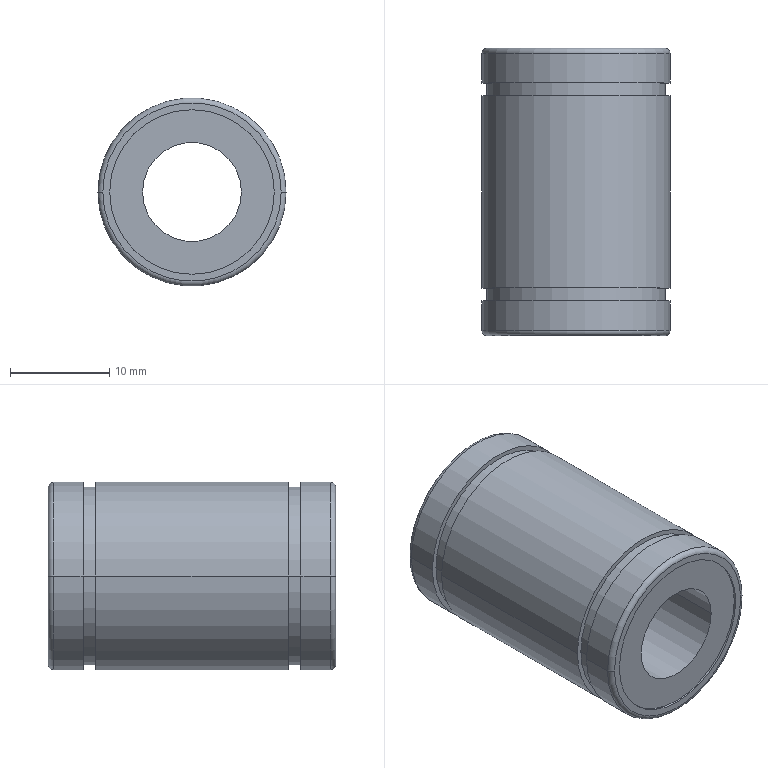Part | NX | 1 solid | 28 faces | box 19 x 29 x 19 mm | volume 5808 mm3 | cylinder 16 | plane 8 | torus 4 | commonest cylinder face diameters 19 x6 16.6 x4 18 x4 10 x2
STEP:
#1=CARTESIAN_POINT('',(-5.,-14.3,0.));
#2=VERTEX_POINT('',#1);
#3=CARTESIAN_POINT('',(5.,-14.3,0.));
#4=VERTEX_POINT('',#3);
#5=CARTESIAN_POINT('',(0.,-14.3,0.));
#6=DIRECTION('',(0.,1.,0.));
#7=DIRECTION('',(-1.,0.,0.));
#8=AXIS2_PLACEMENT_3D('',#5,#6,#7);
#9=CIRCLE('',#8,5.);
#10=EDGE_CURVE('',#2,#4,#9,.T.);
#11=ORIENTED_EDGE('',*,*,#10,.F.);
#12=CARTESIAN_POINT('',(-5.,14.3,0.));
#13=VERTEX_POINT('',#12);
#14=CARTESIAN_POINT('',(-5.,-15.95,0.));
#15=DIRECTION('',(0.,1.,0.));
#16=VECTOR('',#15,1000.);
#17=LINE('',#14,#16);
#18=EDGE_CURVE('',#2,#13,#17,.T.);
#19=ORIENTED_EDGE('',*,*,#18,.T.);
#20=CARTESIAN_POINT('',(5.,14.3,0.));
#21=VERTEX_POINT('',#20);
#22=CARTESIAN_POINT('',(0.,14.3,0.));
#23=DIRECTION('',(0.,-1.,0.));
#24=DIRECTION('',(1.,0.,0.));
#25=AXIS2_PLACEMENT_3D('',#22,#23,#24);
#26=CIRCLE('',#25,5.);
#27=EDGE_CURVE('',#21,#13,#26,.T.);
#28=ORIENTED_EDGE('',*,*,#27,.F.);
#29=CARTESIAN_POINT('',(5.,-15.95,0.));
#30=DIRECTION('',(0.,1.,0.));
#31=VECTOR('',#30,1000.);
#32=LINE('',#29,#31);
#33=EDGE_CURVE('',#4,#21,#32,.T.);
#34=ORIENTED_EDGE('',*,*,#33,.F.);
#35=EDGE_LOOP('',(#11,#19,#28,#34));
#36=FACE_BOUND('',#35,.T.);
#37=CARTESIAN_POINT('',(0.,-15.95,0.));
#38=DIRECTION('',(0.,1.,0.));
#39=DIRECTION('',(1.,0.,0.));
#40=AXIS2_PLACEMENT_3D('',#37,#38,#39);
#41=CYLINDRICAL_SURFACE('',#40,5.);
#42=ADVANCED_FACE('',(#36),#41,.F.);
#43=CARTESIAN_POINT('',(-8.3,14.3,0.));
#44=VERTEX_POINT('',#43);
#45=CARTESIAN_POINT('',(8.3,14.3,0.));
#46=VERTEX_POINT('',#45);
#47=CARTESIAN_POINT('',(0.,14.3,0.));
#48=DIRECTION('',(0.,1.,0.));
#49=DIRECTION('',(1.,0.,0.));
#50=AXIS2_PLACEMENT_3D('',#47,#48,#49);
#51=CIRCLE('',#50,8.3);
#52=EDGE_CURVE('',#44,#46,#51,.T.);
#53=ORIENTED_EDGE('',*,*,#52,.T.);
#54=CARTESIAN_POINT('',(0.,14.3,0.));
#55=DIRECTION('',(0.,1.,0.));
#56=DIRECTION('',(1.,0.,0.));
#57=AXIS2_PLACEMENT_3D('',#54,#55,#56);
#58=CIRCLE('',#57,8.3);
#59=EDGE_CURVE('',#46,#44,#58,.T.);
#60=ORIENTED_EDGE('',*,*,#59,.T.);
#61=EDGE_LOOP('',(#53,#60));
#62=FACE_BOUND('',#61,.T.);
#63=ORIENTED_EDGE('',*,*,#27,.T.);
#64=CARTESIAN_POINT('',(0.,14.3,0.));
#65=DIRECTION('',(0.,-1.,0.));
#66=DIRECTION('',(1.,0.,0.));
#67=AXIS2_PLACEMENT_3D('',#64,#65,#66);
#68=CIRCLE('',#67,5.);
#69=EDGE_CURVE('',#13,#21,#68,.T.);
#70=ORIENTED_EDGE('',*,*,#69,.T.);
#71=EDGE_LOOP('',(#63,#70));
#72=FACE_BOUND('',#71,.T.);
#73=CARTESIAN_POINT('',(0.,14.3,0.));
#74=DIRECTION('',(0.,1.,0.));
#75=DIRECTION('',(1.,0.,0.));
#76=AXIS2_PLACEMENT_3D('',#73,#74,#75);
#77=PLANE('',#76);
#78=ADVANCED_FACE('',(#62,#72),#77,.T.);
#79=ORIENTED_EDGE('',*,*,#52,.F.);
#80=CARTESIAN_POINT('',(-8.3,14.5,0.));
#81=VERTEX_POINT('',#80);
#82=CARTESIAN_POINT('',(-8.3,14.5,0.));
#83=DIRECTION('',(0.,-1.,0.));
#84=VECTOR('',#83,1000.);
#85=LINE('',#82,#84);
#86=EDGE_CURVE('',#44,#81,#85,.F.);
#87=ORIENTED_EDGE('',*,*,#86,.T.);
#88=CARTESIAN_POINT('',(8.3,14.5,0.));
#89=VERTEX_POINT('',#88);
#90=CARTESIAN_POINT('',(0.,14.5,0.));
#91=DIRECTION('',(0.,-1.,0.));
#92=DIRECTION('',(-1.,0.,0.));
#93=AXIS2_PLACEMENT_3D('',#90,#91,#92);
#94=CIRCLE('',#93,8.3);
#95=EDGE_CURVE('',#89,#81,#94,.T.);
#96=ORIENTED_EDGE('',*,*,#95,.F.);
#97=CARTESIAN_POINT('',(8.3,14.5,0.));
#98=DIRECTION('',(0.,-1.,0.));
#99=VECTOR('',#98,1000.);
#100=LINE('',#97,#99);
#101=EDGE_CURVE('',#46,#89,#100,.F.);
#102=ORIENTED_EDGE('',*,*,#101,.F.);
#103=EDGE_LOOP('',(#79,#87,#96,#102));
#104=FACE_BOUND('',#103,.T.);
#105=CARTESIAN_POINT('',(0.,14.5,0.));
#106=DIRECTION('',(0.,-1.,0.));
#107=DIRECTION('',(-1.,0.,0.));
#108=AXIS2_PLACEMENT_3D('',#105,#106,#107);
#109=CYLINDRICAL_SURFACE('',#108,8.3);
#110=ADVANCED_FACE('',(#104),#109,.F.);
#111=CARTESIAN_POINT('',(-9.,14.5,0.));
#112=VERTEX_POINT('',#111);
#113=CARTESIAN_POINT('',(9.,14.5,0.));
#114=VERTEX_POINT('',#113);
#115=CARTESIAN_POINT('',(0.,14.5,0.));
#116=DIRECTION('',(0.,-1.,0.));
#117=DIRECTION('',(1.,0.,0.));
#118=AXIS2_PLACEMENT_3D('',#115,#116,#117);
#119=CIRCLE('',#118,9.);
#120=EDGE_CURVE('',#112,#114,#119,.T.);
#121=ORIENTED_EDGE('',*,*,#120,.F.);
#122=CARTESIAN_POINT('',(0.,14.5,0.));
#123=DIRECTION('',(0.,-1.,0.));
#124=DIRECTION('',(1.,0.,0.));
#125=AXIS2_PLACEMENT_3D('',#122,#123,#124);
#126=CIRCLE('',#125,9.);
#127=EDGE_CURVE('',#114,#112,#126,.T.);
#128=ORIENTED_EDGE('',*,*,#127,.F.);
#129=EDGE_LOOP('',(#121,#128));
#130=FACE_BOUND('',#129,.T.);
#131=CARTESIAN_POINT('',(0.,14.5,0.));
#132=DIRECTION('',(0.,-1.,0.));
#133=DIRECTION('',(-1.,0.,0.));
#134=AXIS2_PLACEMENT_3D('',#131,#132,#133);
#135=CIRCLE('',#134,8.3);
#136=EDGE_CURVE('',#81,#89,#135,.T.);
#137=ORIENTED_EDGE('',*,*,#136,.T.);
#138=ORIENTED_EDGE('',*,*,#95,.T.);
#139=EDGE_LOOP('',(#137,#138));
#140=FACE_BOUND('',#139,.T.);
#141=CARTESIAN_POINT('',(0.,14.5,0.));
#142=DIRECTION('',(0.,-1.,0.));
#143=DIRECTION('',(0.,0.,-1.));
#144=AXIS2_PLACEMENT_3D('',#141,#142,#143);
#145=PLANE('',#144);
#146=ADVANCED_FACE('',(#130,#140),#145,.F.);
#147=CARTESIAN_POINT('',(-9.5,14.,0.));
#148=VERTEX_POINT('',#147);
#149=CARTESIAN_POINT('',(9.5,14.,0.));
#150=VERTEX_POINT('',#149);
#151=CARTESIAN_POINT('',(0.,14.,0.));
#152=DIRECTION('',(0.,-1.,0.));
#153=DIRECTION('',(1.,0.,0.));
#154=AXIS2_PLACEMENT_3D('',#151,#152,#153);
#155=CIRCLE('',#154,9.5);
#156=EDGE_CURVE('',#148,#150,#155,.T.);
#157=ORIENTED_EDGE('',*,*,#156,.F.);
#158=CARTESIAN_POINT('',(-9.,14.,0.));
#159=DIRECTION('',(0.,0.,1.));
#160=DIRECTION('',(-1.,0.,0.));
#161=AXIS2_PLACEMENT_3D('',#158,#159,#160);
#162=CIRCLE('',#161,0.5);
#163=EDGE_CURVE('',#112,#148,#162,.T.);
#164=ORIENTED_EDGE('',*,*,#163,.F.);
#165=ORIENTED_EDGE('',*,*,#120,.T.);
#166=CARTESIAN_POINT('',(9.,14.,0.));
#167=DIRECTION('',(0.,0.,-1.));
#168=DIRECTION('',(1.,0.,0.));
#169=AXIS2_PLACEMENT_3D('',#166,#167,#168);
#170=CIRCLE('',#169,0.5);
#171=EDGE_CURVE('',#114,#150,#170,.T.);
#172=ORIENTED_EDGE('',*,*,#171,.T.);
#173=EDGE_LOOP('',(#157,#164,#165,#172));
#174=FACE_BOUND('',#173,.T.);
#175=CARTESIAN_POINT('',(0.,14.,0.));
#176=DIRECTION('',(0.,-1.,0.));
#177=DIRECTION('',(1.,0.,0.));
#178=AXIS2_PLACEMENT_3D('',#175,#176,#177);
#179=TOROIDAL_SURFACE('',#178,9.,0.5);
#180=ADVANCED_FACE('',(#174),#179,.T.);
#181=ORIENTED_EDGE('',*,*,#156,.T.);
#182=CARTESIAN_POINT('',(9.5,11.,0.));
#183=VERTEX_POINT('',#182);
#184=CARTESIAN_POINT('',(9.5,-15.95,0.));
#185=DIRECTION('',(0.,1.,0.));
#186=VECTOR('',#185,1000.);
#187=LINE('',#184,#186);
#188=EDGE_CURVE('',#183,#150,#187,.T.);
#189=ORIENTED_EDGE('',*,*,#188,.F.);
#190=CARTESIAN_POINT('',(-9.5,11.,0.));
#191=VERTEX_POINT('',#190);
#192=CARTESIAN_POINT('',(0.,11.,0.));
#193=DIRECTION('',(0.,-1.,0.));
#194=DIRECTION('',(-1.,0.,0.));
#195=AXIS2_PLACEMENT_3D('',#192,#193,#194);
#196=CIRCLE('',#195,9.5);
#197=EDGE_CURVE('',#191,#183,#196,.T.);
#198=ORIENTED_EDGE('',*,*,#197,.F.);
#199=CARTESIAN_POINT('',(-9.5,-15.95,0.));
#200=DIRECTION('',(0.,1.,0.));
#201=VECTOR('',#200,1000.);
#202=LINE('',#199,#201);
#203=EDGE_CURVE('',#191,#148,#202,.T.);
#204=ORIENTED_EDGE('',*,*,#203,.T.);
#205=EDGE_LOOP('',(#181,#189,#198,#204));
#206=FACE_BOUND('',#205,.T.);
#207=CARTESIAN_POINT('',(0.,-15.95,0.));
#208=DIRECTION('',(0.,1.,0.));
#209=DIRECTION('',(1.,0.,0.));
#210=AXIS2_PLACEMENT_3D('',#207,#208,#209);
#211=CYLINDRICAL_SURFACE('',#210,9.5);
#212=ADVANCED_FACE('',(#206),#211,.T.);
#213=CARTESIAN_POINT('',(-8.3,-14.3,0.));
#214=VERTEX_POINT('',#213);
#215=CARTESIAN_POINT('',(8.3,-14.3,0.));
#216=VERTEX_POINT('',#215);
#217=CARTESIAN_POINT('',(0.,-14.3,0.));
#218=DIRECTION('',(0.,-1.,0.));
#219=DIRECTION('',(1.,0.,0.));
#220=AXIS2_PLACEMENT_3D('',#217,#218,#219);
#221=CIRCLE('',#220,8.3);
#222=EDGE_CURVE('',#214,#216,#221,.T.);
#223=ORIENTED_EDGE('',*,*,#222,.T.);
#224=CARTESIAN_POINT('',(0.,-14.3,0.));
#225=DIRECTION('',(0.,-1.,0.));
#226=DIRECTION('',(1.,0.,0.));
#227=AXIS2_PLACEMENT_3D('',#224,#225,#226);
#228=CIRCLE('',#227,8.3);
#229=EDGE_CURVE('',#216,#214,#228,.T.);
#230=ORIENTED_EDGE('',*,*,#229,.T.);
#231=EDGE_LOOP('',(#223,#230));
#232=FACE_BOUND('',#231,.T.);
#233=ORIENTED_EDGE('',*,*,#10,.T.);
#234=CARTESIAN_POINT('',(0.,-14.3,0.));
#235=DIRECTION('',(0.,1.,0.));
#236=DIRECTION('',(-1.,0.,0.));
#237=AXIS2_PLACEMENT_3D('',#234,#235,#236);
#238=CIRCLE('',#237,5.);
#239=EDGE_CURVE('',#4,#2,#238,.T.);
#240=ORIENTED_EDGE('',*,*,#239,.T.);
#241=EDGE_LOOP('',(#233,#240));
#242=FACE_BOUND('',#241,.T.);
#243=CARTESIAN_POINT('',(0.,-14.3,0.));
#244=DIRECTION('',(0.,1.,0.));
#245=DIRECTION('',(1.,0.,0.));
#246=AXIS2_PLACEMENT_3D('',#243,#244,#245);
#247=PLANE('',#246);
#248=ADVANCED_FACE('',(#232,#242),#247,.F.);
#249=CARTESIAN_POINT('',(-9.,-14.5,0.));
#250=VERTEX_POINT('',#249);
#251=CARTESIAN_POINT('',(9.,-14.5,0.));
#252=VERTEX_POINT('',#251);
#253=CARTESIAN_POINT('',(0.,-14.5,0.));
#254=DIRECTION('',(0.,-1.,0.));
#255=DIRECTION('',(1.,0.,0.008751));
#256=AXIS2_PLACEMENT_3D('',#253,#254,#255);
#257=CIRCLE('',#256,9.);
#258=EDGE_CURVE('',#250,#252,#257,.T.);
#259=ORIENTED_EDGE('',*,*,#258,.T.);
#260=CARTESIAN_POINT('',(0.,-14.5,0.));
#261=DIRECTION('',(0.,-1.,0.));
#262=DIRECTION('',(1.,0.,0.008751));
#263=AXIS2_PLACEMENT_3D('',#260,#261,#262);
#264=CIRCLE('',#263,9.);
#265=EDGE_CURVE('',#252,#250,#264,.T.);
#266=ORIENTED_EDGE('',*,*,#265,.T.);
#267=EDGE_LOOP('',(#259,#266));
#268=FACE_BOUND('',#267,.T.);
#269=CARTESIAN_POINT('',(-8.3,-14.5,0.));
#270=VERTEX_POINT('',#269);
#271=CARTESIAN_POINT('',(8.3,-14.5,0.));
#272=VERTEX_POINT('',#271);
#273=CARTESIAN_POINT('',(0.,-14.5,0.));
#274=DIRECTION('',(0.,1.,0.));
#275=DIRECTION('',(1.,0.,0.));
#276=AXIS2_PLACEMENT_3D('',#273,#274,#275);
#277=CIRCLE('',#276,8.3);
#278=EDGE_CURVE('',#270,#272,#277,.T.);
#279=ORIENTED_EDGE('',*,*,#278,.T.);
#280=CARTESIAN_POINT('',(0.,-14.5,0.));
#281=DIRECTION('',(0.,1.,0.));
#282=DIRECTION('',(1.,0.,0.));
#283=AXIS2_PLACEMENT_3D('',#280,#281,#282);
#284=CIRCLE('',#283,8.3);
#285=EDGE_CURVE('',#272,#270,#284,.T.);
#286=ORIENTED_EDGE('',*,*,#285,.T.);
#287=EDGE_LOOP('',(#279,#286));
#288=FACE_BOUND('',#287,.T.);
#289=CARTESIAN_POINT('',(0.,-14.5,0.));
#290=DIRECTION('',(0.,-1.,0.));
#291=DIRECTION('',(0.,0.,-1.));
#292=AXIS2_PLACEMENT_3D('',#289,#290,#291);
#293=PLANE('',#292);
#294=ADVANCED_FACE('',(#268,#288),#293,.T.);
#295=CARTESIAN_POINT('',(0.,11.,0.));
#296=DIRECTION('',(0.,-1.,0.));
#297=DIRECTION('',(-1.,0.,0.));
#298=AXIS2_PLACEMENT_3D('',#295,#296,#297);
#299=CIRCLE('',#298,9.5);
#300=EDGE_CURVE('',#183,#191,#299,.T.);
#301=ORIENTED_EDGE('',*,*,#300,.T.);
#302=ORIENTED_EDGE('',*,*,#197,.T.);
#303=EDGE_LOOP('',(#301,#302));
#304=FACE_BOUND('',#303,.T.);
#305=CARTESIAN_POINT('',(-9.,11.,0.));
#306=VERTEX_POINT('',#305);
#307=CARTESIAN_POINT('',(9.,11.,0.));
#308=VERTEX_POINT('',#307);
#309=CARTESIAN_POINT('',(0.,11.,0.));
#310=DIRECTION('',(0.,1.,0.));
#311=DIRECTION('',(-1.,0.,0.));
#312=AXIS2_PLACEMENT_3D('',#309,#310,#311);
#313=CIRCLE('',#312,9.);
#314=EDGE_CURVE('',#306,#308,#313,.T.);
#315=ORIENTED_EDGE('',*,*,#314,.T.);
#316=CARTESIAN_POINT('',(0.,11.,0.));
#317=DIRECTION('',(0.,1.,0.));
#318=DIRECTION('',(-1.,0.,0.));
#319=AXIS2_PLACEMENT_3D('',#316,#317,#318);
#320=CIRCLE('',#319,9.);
#321=EDGE_CURVE('',#308,#306,#320,.T.);
#322=ORIENTED_EDGE('',*,*,#321,.T.);
#323=EDGE_LOOP('',(#315,#322));
#324=FACE_BOUND('',#323,.T.);
#325=CARTESIAN_POINT('',(0.,11.,0.));
#326=DIRECTION('',(0.,-1.,0.));
#327=DIRECTION('',(0.,0.,-1.));
#328=AXIS2_PLACEMENT_3D('',#325,#326,#327);
#329=PLANE('',#328);
#330=ADVANCED_FACE('',(#304,#324),#329,.T.);
#331=CARTESIAN_POINT('',(9.,9.7,0.));
#332=VERTEX_POINT('',#331);
#333=CARTESIAN_POINT('',(-9.,9.7,0.));
#334=VERTEX_POINT('',#333);
#335=CARTESIAN_POINT('',(0.,9.7,0.));
#336=DIRECTION('',(0.,-1.,0.));
#337=DIRECTION('',(-1.,0.,0.));
#338=AXIS2_PLACEMENT_3D('',#335,#336,#337);
#339=CIRCLE('',#338,9.);
#340=EDGE_CURVE('',#332,#334,#339,.T.);
#341=ORIENTED_EDGE('',*,*,#340,.F.);
#342=CARTESIAN_POINT('',(9.,-15.95,0.));
#343=DIRECTION('',(0.,1.,0.));
#344=VECTOR('',#343,1000.);
#345=LINE('',#342,#344);
#346=EDGE_CURVE('',#332,#308,#345,.T.);
#347=ORIENTED_EDGE('',*,*,#346,.T.);
#348=ORIENTED_EDGE('',*,*,#314,.F.);
#349=CARTESIAN_POINT('',(-9.,-15.95,0.));
#350=DIRECTION('',(0.,1.,0.));
#351=VECTOR('',#350,1000.);
#352=LINE('',#349,#351);
#353=EDGE_CURVE('',#334,#306,#352,.T.);
#354=ORIENTED_EDGE('',*,*,#353,.F.);
#355=EDGE_LOOP('',(#341,#347,#348,#354));
#356=FACE_BOUND('',#355,.T.);
#357=CARTESIAN_POINT('',(0.,-15.95,0.));
#358=DIRECTION('',(0.,1.,0.));
#359=DIRECTION('',(1.,0.,0.));
#360=AXIS2_PLACEMENT_3D('',#357,#358,#359);
#361=CYLINDRICAL_SURFACE('',#360,9.);
#362=ADVANCED_FACE('',(#356),#361,.T.);
#363=CARTESIAN_POINT('',(9.5,-14.,0.));
#364=VERTEX_POINT('',#363);
#365=CARTESIAN_POINT('',(-9.5,-14.,0.));
#366=VERTEX_POINT('',#365);
#367=CARTESIAN_POINT('',(0.,-14.,0.));
#368=DIRECTION('',(0.,-1.,0.));
#369=DIRECTION('',(1.,0.,0.));
#370=AXIS2_PLACEMENT_3D('',#367,#368,#369);
#371=CIRCLE('',#370,9.5);
#372=EDGE_CURVE('',#364,#366,#371,.T.);
#373=ORIENTED_EDGE('',*,*,#372,.T.);
#374=CARTESIAN_POINT('',(-9.,-14.,0.));
#375=DIRECTION('',(0.,0.,1.));
#376=DIRECTION('',(-1.,0.,0.));
#377=AXIS2_PLACEMENT_3D('',#374,#375,#376);
#378=CIRCLE('',#377,0.5);
#379=EDGE_CURVE('',#250,#366,#378,.F.);
#380=ORIENTED_EDGE('',*,*,#379,.F.);
#381=ORIENTED_EDGE('',*,*,#265,.F.);
#382=CARTESIAN_POINT('',(9.,-14.,0.));
#383=DIRECTION('',(0.,0.,-1.));
#384=DIRECTION('',(1.,0.,0.));
#385=AXIS2_PLACEMENT_3D('',#382,#383,#384);
#386=CIRCLE('',#385,0.5);
#387=EDGE_CURVE('',#252,#364,#386,.F.);
#388=ORIENTED_EDGE('',*,*,#387,.T.);
#389=EDGE_LOOP('',(#373,#380,#381,#388));
#390=FACE_BOUND('',#389,.T.);
#391=CARTESIAN_POINT('',(0.,-14.,0.));
#392=DIRECTION('',(0.,-1.,0.));
#393=DIRECTION('',(1.,0.,0.));
#394=AXIS2_PLACEMENT_3D('',#391,#392,#393);
#395=TOROIDAL_SURFACE('',#394,9.,0.5);
#396=ADVANCED_FACE('',(#390),#395,.T.);
#397=CARTESIAN_POINT('',(9.5,9.7,0.));
#398=VERTEX_POINT('',#397);
#399=CARTESIAN_POINT('',(-9.5,9.7,0.));
#400=VERTEX_POINT('',#399);
#401=CARTESIAN_POINT('',(0.,9.7,0.));
#402=DIRECTION('',(0.,1.,0.));
#403=DIRECTION('',(-1.,0.,0.));
#404=AXIS2_PLACEMENT_3D('',#401,#402,#403);
#405=CIRCLE('',#404,9.5);
#406=EDGE_CURVE('',#398,#400,#405,.T.);
#407=ORIENTED_EDGE('',*,*,#406,.T.);
#408=CARTESIAN_POINT('',(0.,9.7,0.));
#409=DIRECTION('',(0.,1.,0.));
#410=DIRECTION('',(-1.,0.,0.));
#411=AXIS2_PLACEMENT_3D('',#408,#409,#410);
#412=CIRCLE('',#411,9.5);
#413=EDGE_CURVE('',#400,#398,#412,.T.);
#414=ORIENTED_EDGE('',*,*,#413,.T.);
#415=EDGE_LOOP('',(#407,#414));
#416=FACE_BOUND('',#415,.T.);
#417=ORIENTED_EDGE('',*,*,#340,.T.);
#418=CARTESIAN_POINT('',(0.,9.7,0.));
#419=DIRECTION('',(0.,-1.,0.));
#420=DIRECTION('',(-1.,0.,0.));
#421=AXIS2_PLACEMENT_3D('',#418,#419,#420);
#422=CIRCLE('',#421,9.);
#423=EDGE_CURVE('',#334,#332,#422,.T.);
#424=ORIENTED_EDGE('',*,*,#423,.T.);
#425=EDGE_LOOP('',(#417,#424));
#426=FACE_BOUND('',#425,.T.);
#427=CARTESIAN_POINT('',(0.,9.7,0.));
#428=DIRECTION('',(0.,-1.,0.));
#429=DIRECTION('',(0.,0.,-1.));
#430=AXIS2_PLACEMENT_3D('',#427,#428,#429);
#431=PLANE('',#430);
#432=ADVANCED_FACE('',(#416,#426),#431,.F.);
#433=ORIENTED_EDGE('',*,*,#406,.F.);
#434=CARTESIAN_POINT('',(9.5,-9.7,0.));
#435=VERTEX_POINT('',#434);
#436=CARTESIAN_POINT('',(9.5,-15.95,0.));
#437=DIRECTION('',(0.,1.,0.));
#438=VECTOR('',#437,1000.);
#439=LINE('',#436,#438);
#440=EDGE_CURVE('',#435,#398,#439,.T.);
#441=ORIENTED_EDGE('',*,*,#440,.F.);
#442=CARTESIAN_POINT('',(-9.5,-9.7,0.));
#443=VERTEX_POINT('',#442);
#444=CARTESIAN_POINT('',(0.,-9.7,0.));
#445=DIRECTION('',(0.,-1.,0.));
#446=DIRECTION('',(-1.,0.,0.));
#447=AXIS2_PLACEMENT_3D('',#444,#445,#446);
#448=CIRCLE('',#447,9.5);
#449=EDGE_CURVE('',#443,#435,#448,.T.);
#450=ORIENTED_EDGE('',*,*,#449,.F.);
#451=CARTESIAN_POINT('',(-9.5,-15.95,0.));
#452=DIRECTION('',(0.,1.,0.));
#453=VECTOR('',#452,1000.);
#454=LINE('',#451,#453);
#455=EDGE_CURVE('',#443,#400,#454,.T.);
#456=ORIENTED_EDGE('',*,*,#455,.T.);
#457=EDGE_LOOP('',(#433,#441,#450,#456));
#458=FACE_BOUND('',#457,.T.);
#459=CARTESIAN_POINT('',(0.,-15.95,0.));
#460=DIRECTION('',(0.,1.,0.));
#461=DIRECTION('',(1.,0.,0.));
#462=AXIS2_PLACEMENT_3D('',#459,#460,#461);
#463=CYLINDRICAL_SURFACE('',#462,9.5);
#464=ADVANCED_FACE('',(#458),#463,.T.);
#465=CARTESIAN_POINT('',(9.5,-11.,0.));
#466=VERTEX_POINT('',#465);
#467=CARTESIAN_POINT('',(-9.5,-11.,0.));
#468=VERTEX_POINT('',#467);
#469=CARTESIAN_POINT('',(0.,-11.,0.));
#470=DIRECTION('',(0.,1.,0.));
#471=DIRECTION('',(-1.,0.,0.));
#472=AXIS2_PLACEMENT_3D('',#469,#470,#471);
#473=CIRCLE('',#472,9.5);
#474=EDGE_CURVE('',#466,#468,#473,.T.);
#475=ORIENTED_EDGE('',*,*,#474,.F.);
#476=CARTESIAN_POINT('',(9.5,-15.95,0.));
#477=DIRECTION('',(0.,1.,0.));
#478=VECTOR('',#477,1000.);
#479=LINE('',#476,#478);
#480=EDGE_CURVE('',#364,#466,#479,.T.);
#481=ORIENTED_EDGE('',*,*,#480,.F.);
#482=CARTESIAN_POINT('',(0.,-14.,0.));
#483=DIRECTION('',(0.,-1.,0.));
#484=DIRECTION('',(1.,0.,0.));
#485=AXIS2_PLACEMENT_3D('',#482,#483,#484);
#486=CIRCLE('',#485,9.5);
#487=EDGE_CURVE('',#366,#364,#486,.T.);
#488=ORIENTED_EDGE('',*,*,#487,.F.);
#489=CARTESIAN_POINT('',(-9.5,-15.95,0.));
#490=DIRECTION('',(0.,1.,0.));
#491=VECTOR('',#490,1000.);
#492=LINE('',#489,#491);
#493=EDGE_CURVE('',#366,#468,#492,.T.);
#494=ORIENTED_EDGE('',*,*,#493,.T.);
#495=EDGE_LOOP('',(#475,#481,#488,#494));
#496=FACE_BOUND('',#495,.T.);
#497=CARTESIAN_POINT('',(0.,-15.95,0.));
#498=DIRECTION('',(0.,1.,0.));
#499=DIRECTION('',(1.,0.,0.));
#500=AXIS2_PLACEMENT_3D('',#497,#498,#499);
#501=CYLINDRICAL_SURFACE('',#500,9.5);
#502=ADVANCED_FACE('',(#496),#501,.T.);
#503=ORIENTED_EDGE('',*,*,#449,.T.);
#504=CARTESIAN_POINT('',(0.,-9.7,0.));
#505=DIRECTION('',(0.,-1.,0.));
#506=DIRECTION('',(-1.,0.,0.));
#507=AXIS2_PLACEMENT_3D('',#504,#505,#506);
#508=CIRCLE('',#507,9.5);
#509=EDGE_CURVE('',#435,#443,#508,.T.);
#510=ORIENTED_EDGE('',*,*,#509,.T.);
#511=EDGE_LOOP('',(#503,#510));
#512=FACE_BOUND('',#511,.T.);
#513=CARTESIAN_POINT('',(-9.,-9.7,0.));
#514=VERTEX_POINT('',#513);
#515=CARTESIAN_POINT('',(9.,-9.7,0.));
#516=VERTEX_POINT('',#515);
#517=CARTESIAN_POINT('',(0.,-9.7,0.));
#518=DIRECTION('',(0.,1.,0.));
#519=DIRECTION('',(-1.,0.,0.));
#520=AXIS2_PLACEMENT_3D('',#517,#518,#519);
#521=CIRCLE('',#520,9.);
#522=EDGE_CURVE('',#514,#516,#521,.T.);
#523=ORIENTED_EDGE('',*,*,#522,.T.);
#524=CARTESIAN_POINT('',(0.,-9.7,0.));
#525=DIRECTION('',(0.,1.,0.));
#526=DIRECTION('',(-1.,0.,0.));
#527=AXIS2_PLACEMENT_3D('',#524,#525,#526);
#528=CIRCLE('',#527,9.);
#529=EDGE_CURVE('',#516,#514,#528,.T.);
#530=ORIENTED_EDGE('',*,*,#529,.T.);
#531=EDGE_LOOP('',(#523,#530));
#532=FACE_BOUND('',#531,.T.);
#533=CARTESIAN_POINT('',(0.,-9.7,0.));
#534=DIRECTION('',(0.,-1.,0.));
#535=DIRECTION('',(0.,0.,-1.));
#536=AXIS2_PLACEMENT_3D('',#533,#534,#535);
#537=PLANE('',#536);
#538=ADVANCED_FACE('',(#512,#532),#537,.T.);
#539=ORIENTED_EDGE('',*,*,#522,.F.);
#540=CARTESIAN_POINT('',(-9.,-11.,0.));
#541=VERTEX_POINT('',#540);
#542=CARTESIAN_POINT('',(-9.,-15.95,0.));
#543=DIRECTION('',(0.,1.,0.));
#544=VECTOR('',#543,1000.);
#545=LINE('',#542,#544);
#546=EDGE_CURVE('',#514,#541,#545,.F.);
#547=ORIENTED_EDGE('',*,*,#546,.T.);
#548=CARTESIAN_POINT('',(9.,-11.,0.));
#549=VERTEX_POINT('',#548);
#550=CARTESIAN_POINT('',(0.,-11.,0.));
#551=DIRECTION('',(0.,-1.,0.));
#552=DIRECTION('',(-1.,0.,0.));
#553=AXIS2_PLACEMENT_3D('',#550,#551,#552);
#554=CIRCLE('',#553,9.);
#555=EDGE_CURVE('',#549,#541,#554,.T.);
#556=ORIENTED_EDGE('',*,*,#555,.F.);
#557=CARTESIAN_POINT('',(9.,-15.95,0.));
#558=DIRECTION('',(0.,1.,0.));
#559=VECTOR('',#558,1000.);
#560=LINE('',#557,#559);
#561=EDGE_CURVE('',#516,#549,#560,.F.);
#562=ORIENTED_EDGE('',*,*,#561,.F.);
#563=EDGE_LOOP('',(#539,#547,#556,#562));
#564=FACE_BOUND('',#563,.T.);
#565=CARTESIAN_POINT('',(0.,-15.95,0.));
#566=DIRECTION('',(0.,1.,0.));
#567=DIRECTION('',(1.,0.,0.));
#568=AXIS2_PLACEMENT_3D('',#565,#566,#567);
#569=CYLINDRICAL_SURFACE('',#568,9.);
#570=ADVANCED_FACE('',(#564),#569,.T.);
#571=ORIENTED_EDGE('',*,*,#278,.F.);
#572=CARTESIAN_POINT('',(-8.3,-14.5,0.));
#573=DIRECTION('',(0.,-1.,0.));
#574=VECTOR('',#573,1000.);
#575=LINE('',#572,#574);
#576=EDGE_CURVE('',#270,#214,#575,.F.);
#577=ORIENTED_EDGE('',*,*,#576,.T.);
#578=ORIENTED_EDGE('',*,*,#229,.F.);
#579=CARTESIAN_POINT('',(8.3,-14.5,0.));
#580=DIRECTION('',(0.,-1.,0.));
#581=VECTOR('',#580,1000.);
#582=LINE('',#579,#581);
#583=EDGE_CURVE('',#272,#216,#582,.F.);
#584=ORIENTED_EDGE('',*,*,#583,.F.);
#585=EDGE_LOOP('',(#571,#577,#578,#584));
#586=FACE_BOUND('',#585,.T.);
#587=CARTESIAN_POINT('',(0.,-14.5,0.));
#588=DIRECTION('',(0.,-1.,0.));
#589=DIRECTION('',(-1.,0.,0.));
#590=AXIS2_PLACEMENT_3D('',#587,#588,#589);
#591=CYLINDRICAL_SURFACE('',#590,8.3);
#592=ADVANCED_FACE('',(#586),#591,.F.);
#593=ORIENTED_EDGE('',*,*,#474,.T.);
#594=CARTESIAN_POINT('',(0.,-11.,0.));
#595=DIRECTION('',(0.,1.,0.));
#596=DIRECTION('',(-1.,0.,0.));
#597=AXIS2_PLACEMENT_3D('',#594,#595,#596);
#598=CIRCLE('',#597,9.5);
#599=EDGE_CURVE('',#468,#466,#598,.T.);
#600=ORIENTED_EDGE('',*,*,#599,.T.);
#601=EDGE_LOOP('',(#593,#600));
#602=FACE_BOUND('',#601,.T.);
#603=CARTESIAN_POINT('',(0.,-11.,0.));
#604=DIRECTION('',(0.,-1.,0.));
#605=DIRECTION('',(-1.,0.,0.));
#606=AXIS2_PLACEMENT_3D('',#603,#604,#605);
#607=CIRCLE('',#606,9.);
#608=EDGE_CURVE('',#541,#549,#607,.T.);
#609=ORIENTED_EDGE('',*,*,#608,.T.);
#610=ORIENTED_EDGE('',*,*,#555,.T.);
#611=EDGE_LOOP('',(#609,#610));
#612=FACE_BOUND('',#611,.T.);
#613=CARTESIAN_POINT('',(0.,-11.,0.));
#614=DIRECTION('',(0.,-1.,0.));
#615=DIRECTION('',(0.,0.,-1.));
#616=AXIS2_PLACEMENT_3D('',#613,#614,#615);
#617=PLANE('',#616);
#618=ADVANCED_FACE('',(#602,#612),#617,.F.);
#619=ORIENTED_EDGE('',*,*,#33,.T.);
#620=ORIENTED_EDGE('',*,*,#69,.F.);
#621=ORIENTED_EDGE('',*,*,#18,.F.);
#622=ORIENTED_EDGE('',*,*,#239,.F.);
#623=EDGE_LOOP('',(#619,#620,#621,#622));
#624=FACE_BOUND('',#623,.T.);
#625=CARTESIAN_POINT('',(0.,-15.95,0.));
#626=DIRECTION('',(0.,1.,0.));
#627=DIRECTION('',(1.,0.,0.));
#628=AXIS2_PLACEMENT_3D('',#625,#626,#627);
#629=CYLINDRICAL_SURFACE('',#628,5.);
#630=ADVANCED_FACE('',(#624),#629,.F.);
#631=ORIENTED_EDGE('',*,*,#608,.F.);
#632=ORIENTED_EDGE('',*,*,#546,.F.);
#633=ORIENTED_EDGE('',*,*,#529,.F.);
#634=ORIENTED_EDGE('',*,*,#561,.T.);
#635=EDGE_LOOP('',(#631,#632,#633,#634));
#636=FACE_BOUND('',#635,.T.);
#637=CARTESIAN_POINT('',(0.,-15.95,0.));
#638=DIRECTION('',(0.,1.,0.));
#639=DIRECTION('',(1.,0.,0.));
#640=AXIS2_PLACEMENT_3D('',#637,#638,#639);
#641=CYLINDRICAL_SURFACE('',#640,9.);
#642=ADVANCED_FACE('',(#636),#641,.T.);
#643=ORIENTED_EDGE('',*,*,#346,.F.);
#644=ORIENTED_EDGE('',*,*,#423,.F.);
#645=ORIENTED_EDGE('',*,*,#353,.T.);
#646=ORIENTED_EDGE('',*,*,#321,.F.);
#647=EDGE_LOOP('',(#643,#644,#645,#646));
#648=FACE_BOUND('',#647,.T.);
#649=CARTESIAN_POINT('',(0.,-15.95,0.));
#650=DIRECTION('',(0.,1.,0.));
#651=DIRECTION('',(1.,0.,0.));
#652=AXIS2_PLACEMENT_3D('',#649,#650,#651);
#653=CYLINDRICAL_SURFACE('',#652,9.);
#654=ADVANCED_FACE('',(#648),#653,.T.);
#655=ORIENTED_EDGE('',*,*,#372,.F.);
#656=ORIENTED_EDGE('',*,*,#480,.T.);
#657=ORIENTED_EDGE('',*,*,#599,.F.);
#658=ORIENTED_EDGE('',*,*,#493,.F.);
#659=EDGE_LOOP('',(#655,#656,#657,#658));
#660=FACE_BOUND('',#659,.T.);
#661=CARTESIAN_POINT('',(0.,-15.95,0.));
#662=DIRECTION('',(0.,1.,0.));
#663=DIRECTION('',(1.,0.,0.));
#664=AXIS2_PLACEMENT_3D('',#661,#662,#663);
#665=CYLINDRICAL_SURFACE('',#664,9.5);
#666=ADVANCED_FACE('',(#660),#665,.T.);
#667=ORIENTED_EDGE('',*,*,#222,.F.);
#668=ORIENTED_EDGE('',*,*,#576,.F.);
#669=ORIENTED_EDGE('',*,*,#285,.F.);
#670=ORIENTED_EDGE('',*,*,#583,.T.);
#671=EDGE_LOOP('',(#667,#668,#669,#670));
#672=FACE_BOUND('',#671,.T.);
#673=CARTESIAN_POINT('',(0.,-14.5,0.));
#674=DIRECTION('',(0.,-1.,0.));
#675=DIRECTION('',(-1.,0.,0.));
#676=AXIS2_PLACEMENT_3D('',#673,#674,#675);
#677=CYLINDRICAL_SURFACE('',#676,8.3);
#678=ADVANCED_FACE('',(#672),#677,.F.);
#679=ORIENTED_EDGE('',*,*,#136,.F.);
#680=ORIENTED_EDGE('',*,*,#86,.F.);
#681=ORIENTED_EDGE('',*,*,#59,.F.);
#682=ORIENTED_EDGE('',*,*,#101,.T.);
#683=EDGE_LOOP('',(#679,#680,#681,#682));
#684=FACE_BOUND('',#683,.T.);
#685=CARTESIAN_POINT('',(0.,14.5,0.));
#686=DIRECTION('',(0.,-1.,0.));
#687=DIRECTION('',(-1.,0.,0.));
#688=AXIS2_PLACEMENT_3D('',#685,#686,#687);
#689=CYLINDRICAL_SURFACE('',#688,8.3);
#690=ADVANCED_FACE('',(#684),#689,.F.);
#691=ORIENTED_EDGE('',*,*,#300,.F.);
#692=ORIENTED_EDGE('',*,*,#188,.T.);
#693=CARTESIAN_POINT('',(0.,14.,0.));
#694=DIRECTION('',(0.,-1.,0.));
#695=DIRECTION('',(1.,0.,0.));
#696=AXIS2_PLACEMENT_3D('',#693,#694,#695);
#697=CIRCLE('',#696,9.5);
#698=EDGE_CURVE('',#150,#148,#697,.T.);
#699=ORIENTED_EDGE('',*,*,#698,.T.);
#700=ORIENTED_EDGE('',*,*,#203,.F.);
#701=EDGE_LOOP('',(#691,#692,#699,#700));
#702=FACE_BOUND('',#701,.T.);
#703=CARTESIAN_POINT('',(0.,-15.95,0.));
#704=DIRECTION('',(0.,1.,0.));
#705=DIRECTION('',(1.,0.,0.));
#706=AXIS2_PLACEMENT_3D('',#703,#704,#705);
#707=CYLINDRICAL_SURFACE('',#706,9.5);
#708=ADVANCED_FACE('',(#702),#707,.T.);
#709=ORIENTED_EDGE('',*,*,#440,.T.);
#710=ORIENTED_EDGE('',*,*,#413,.F.);
#711=ORIENTED_EDGE('',*,*,#455,.F.);
#712=ORIENTED_EDGE('',*,*,#509,.F.);
#713=EDGE_LOOP('',(#709,#710,#711,#712));
#714=FACE_BOUND('',#713,.T.);
#715=CARTESIAN_POINT('',(0.,-15.95,0.));
#716=DIRECTION('',(0.,1.,0.));
#717=DIRECTION('',(1.,0.,0.));
#718=AXIS2_PLACEMENT_3D('',#715,#716,#717);
#719=CYLINDRICAL_SURFACE('',#718,9.5);
#720=ADVANCED_FACE('',(#714),#719,.T.);
#721=ORIENTED_EDGE('',*,*,#258,.F.);
#722=ORIENTED_EDGE('',*,*,#379,.T.);
#723=ORIENTED_EDGE('',*,*,#487,.T.);
#724=ORIENTED_EDGE('',*,*,#387,.F.);
#725=EDGE_LOOP('',(#721,#722,#723,#724));
#726=FACE_BOUND('',#725,.T.);
#727=CARTESIAN_POINT('',(0.,-14.,0.));
#728=DIRECTION('',(0.,-1.,0.));
#729=DIRECTION('',(1.,0.,0.));
#730=AXIS2_PLACEMENT_3D('',#727,#728,#729);
#731=TOROIDAL_SURFACE('',#730,9.,0.5);
#732=ADVANCED_FACE('',(#726),#731,.T.);
#733=ORIENTED_EDGE('',*,*,#171,.F.);
#734=ORIENTED_EDGE('',*,*,#127,.T.);
#735=ORIENTED_EDGE('',*,*,#163,.T.);
#736=ORIENTED_EDGE('',*,*,#698,.F.);
#737=EDGE_LOOP('',(#733,#734,#735,#736));
#738=FACE_BOUND('',#737,.T.);
#739=CARTESIAN_POINT('',(0.,14.,0.));
#740=DIRECTION('',(0.,-1.,0.));
#741=DIRECTION('',(1.,0.,0.));
#742=AXIS2_PLACEMENT_3D('',#739,#740,#741);
#743=TOROIDAL_SURFACE('',#742,9.,0.5);
#744=ADVANCED_FACE('',(#738),#743,.T.);
#745=CLOSED_SHELL('',(#42,#78,#110,#146,#180,#212,#248,#294,#330,#362,#396,#432,#464,#502,#538,#570,#592,#618,#630,#642,#654,#666,#678,#690,#708,#720,#732,#744));
#746=MANIFOLD_SOLID_BREP('',#745);
#747=(LENGTH_UNIT()NAMED_UNIT(*)SI_UNIT(.MILLI.,.METRE.));
#748=UNCERTAINTY_MEASURE_WITH_UNIT(LENGTH_MEASURE(0.00001),#747,'','');
#749=(NAMED_UNIT(*)PLANE_ANGLE_UNIT()SI_UNIT($,.RADIAN.));
#750=(NAMED_UNIT(*)SI_UNIT($,.STERADIAN.)SOLID_ANGLE_UNIT());
#751=(GEOMETRIC_REPRESENTATION_CONTEXT(3)GLOBAL_UNCERTAINTY_ASSIGNED_CONTEXT((#748))GLOBAL_UNIT_ASSIGNED_CONTEXT((#747,#749,#750))REPRESENTATION_CONTEXT('',''));
#752=ADVANCED_BREP_SHAPE_REPRESENTATION('',(#746),#751);